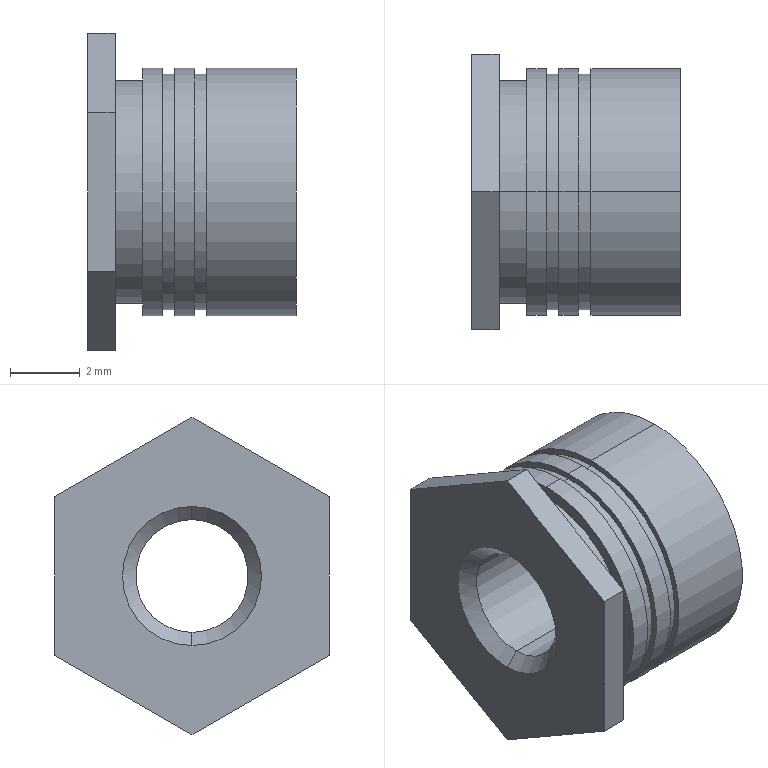Part | NX | features solid 2 | 1 solid | 32 faces | box 6 x 7.9 x 9.122 mm | volume 190.289 mm3 | plane 14 | cylinder 14 | cone 4 | commonest cylinder face diameters 7.12 x6 6.764 x4 3.242 x2 6.408 x2
STEP:
#1=CARTESIAN_POINT('',(-15.92,54.85,-1043.6));
#2=VERTEX_POINT('',#1);
#3=CARTESIAN_POINT('',(-15.92,54.85,-1050.72));
#4=VERTEX_POINT('',#3);
#5=CARTESIAN_POINT('',(-15.92,54.85,-1047.16));
#6=DIRECTION('',(1.,0.,0.));
#7=DIRECTION('',(0.,0.,1.));
#8=AXIS2_PLACEMENT_3D('',#5,#6,#7);
#9=CIRCLE('',#8,3.56);
#10=EDGE_CURVE('',#2,#4,#9,.T.);
#11=ORIENTED_EDGE('',*,*,#10,.F.);
#12=CARTESIAN_POINT('',(-15.92,54.85,-1047.16));
#13=DIRECTION('',(1.,0.,0.));
#14=DIRECTION('',(0.,0.,-1.));
#15=AXIS2_PLACEMENT_3D('',#12,#13,#14);
#16=CIRCLE('',#15,3.56);
#17=EDGE_CURVE('',#4,#2,#16,.T.);
#18=ORIENTED_EDGE('',*,*,#17,.F.);
#19=EDGE_LOOP('',(#11,#18));
#20=FACE_BOUND('',#19,.T.);
#21=CARTESIAN_POINT('',(-15.92,54.85,-1043.956));
#22=VERTEX_POINT('',#21);
#23=CARTESIAN_POINT('',(-15.92,54.85,-1050.364));
#24=VERTEX_POINT('',#23);
#25=CARTESIAN_POINT('',(-15.92,54.85,-1047.16));
#26=DIRECTION('',(-1.,0.,0.));
#27=DIRECTION('',(0.,0.,1.));
#28=AXIS2_PLACEMENT_3D('',#25,#26,#27);
#29=CIRCLE('',#28,3.204);
#30=EDGE_CURVE('',#22,#24,#29,.T.);
#31=ORIENTED_EDGE('',*,*,#30,.F.);
#32=CARTESIAN_POINT('',(-15.92,54.85,-1047.16));
#33=DIRECTION('',(-1.,0.,0.));
#34=DIRECTION('',(0.,0.,-1.));
#35=AXIS2_PLACEMENT_3D('',#32,#33,#34);
#36=CIRCLE('',#35,3.204);
#37=EDGE_CURVE('',#24,#22,#36,.T.);
#38=ORIENTED_EDGE('',*,*,#37,.F.);
#39=EDGE_LOOP('',(#31,#38));
#40=FACE_BOUND('',#39,.T.);
#41=CARTESIAN_POINT('',(-15.92,54.85,-1045.38));
#42=DIRECTION('',(-1.,0.,0.));
#43=DIRECTION('',(0.,1.,0.));
#44=AXIS2_PLACEMENT_3D('',#41,#42,#43);
#45=PLANE('',#44);
#46=ADVANCED_FACE('',(#20,#40),#45,.T.);
#47=CARTESIAN_POINT('',(-15.35,54.85,-1043.6));
#48=VERTEX_POINT('',#47);
#49=CARTESIAN_POINT('',(-15.35,54.85,-1050.72));
#50=VERTEX_POINT('',#49);
#51=CARTESIAN_POINT('',(-15.35,54.85,-1047.16));
#52=DIRECTION('',(-1.,0.,0.));
#53=DIRECTION('',(0.,0.,1.));
#54=AXIS2_PLACEMENT_3D('',#51,#52,#53);
#55=CIRCLE('',#54,3.56);
#56=EDGE_CURVE('',#48,#50,#55,.T.);
#57=ORIENTED_EDGE('',*,*,#56,.T.);
#58=CARTESIAN_POINT('',(-15.92,54.85,-1050.72));
#59=DIRECTION('',(1.,0.,0.));
#60=VECTOR('',#59,1000.);
#61=LINE('',#58,#60);
#62=EDGE_CURVE('',#4,#50,#61,.T.);
#63=ORIENTED_EDGE('',*,*,#62,.F.);
#64=ORIENTED_EDGE('',*,*,#17,.T.);
#65=CARTESIAN_POINT('',(-15.35,54.85,-1043.6));
#66=DIRECTION('',(-1.,0.,0.));
#67=VECTOR('',#66,1000.);
#68=LINE('',#65,#67);
#69=EDGE_CURVE('',#48,#2,#68,.T.);
#70=ORIENTED_EDGE('',*,*,#69,.F.);
#71=EDGE_LOOP('',(#57,#63,#64,#70));
#72=FACE_BOUND('',#71,.T.);
#73=CARTESIAN_POINT('',(-13.71,54.85,-1047.16));
#74=DIRECTION('',(-1.,0.,0.));
#75=DIRECTION('',(0.,0.,-1.));
#76=AXIS2_PLACEMENT_3D('',#73,#74,#75);
#77=CYLINDRICAL_SURFACE('',#76,3.56);
#78=ADVANCED_FACE('',(#72),#77,.T.);
#79=ORIENTED_EDGE('',*,*,#10,.T.);
#80=ORIENTED_EDGE('',*,*,#62,.T.);
#81=CARTESIAN_POINT('',(-15.35,54.85,-1047.16));
#82=DIRECTION('',(-1.,0.,0.));
#83=DIRECTION('',(0.,0.,-1.));
#84=AXIS2_PLACEMENT_3D('',#81,#82,#83);
#85=CIRCLE('',#84,3.56);
#86=EDGE_CURVE('',#50,#48,#85,.T.);
#87=ORIENTED_EDGE('',*,*,#86,.T.);
#88=ORIENTED_EDGE('',*,*,#69,.T.);
#89=EDGE_LOOP('',(#79,#80,#87,#88));
#90=FACE_BOUND('',#89,.T.);
#91=CARTESIAN_POINT('',(-13.71,54.85,-1047.16));
#92=DIRECTION('',(-1.,0.,0.));
#93=DIRECTION('',(0.,0.,-1.));
#94=AXIS2_PLACEMENT_3D('',#91,#92,#93);
#95=CYLINDRICAL_SURFACE('',#94,3.56);
#96=ADVANCED_FACE('',(#90),#95,.T.);
#97=ORIENTED_EDGE('',*,*,#86,.F.);
#98=ORIENTED_EDGE('',*,*,#56,.F.);
#99=EDGE_LOOP('',(#97,#98));
#100=FACE_BOUND('',#99,.T.);
#101=CARTESIAN_POINT('',(-15.35,54.85,-1043.778));
#102=VERTEX_POINT('',#101);
#103=CARTESIAN_POINT('',(-15.35,54.85,-1050.542));
#104=VERTEX_POINT('',#103);
#105=CARTESIAN_POINT('',(-15.35,54.85,-1047.16));
#106=DIRECTION('',(1.,0.,0.));
#107=DIRECTION('',(0.,0.,1.));
#108=AXIS2_PLACEMENT_3D('',#105,#106,#107);
#109=CIRCLE('',#108,3.382);
#110=EDGE_CURVE('',#102,#104,#109,.T.);
#111=ORIENTED_EDGE('',*,*,#110,.F.);
#112=CARTESIAN_POINT('',(-15.35,54.85,-1047.16));
#113=DIRECTION('',(1.,0.,0.));
#114=DIRECTION('',(0.,0.,-1.));
#115=AXIS2_PLACEMENT_3D('',#112,#113,#114);
#116=CIRCLE('',#115,3.382);
#117=EDGE_CURVE('',#104,#102,#116,.T.);
#118=ORIENTED_EDGE('',*,*,#117,.F.);
#119=EDGE_LOOP('',(#111,#118));
#120=FACE_BOUND('',#119,.T.);
#121=CARTESIAN_POINT('',(-15.35,54.85,-1043.689));
#122=DIRECTION('',(-1.,0.,0.));
#123=DIRECTION('',(0.,1.,0.));
#124=AXIS2_PLACEMENT_3D('',#121,#122,#123);
#125=PLANE('',#124);
#126=ADVANCED_FACE('',(#100,#120),#125,.F.);
#127=CARTESIAN_POINT('',(-14.994,54.85,-1043.778));
#128=VERTEX_POINT('',#127);
#129=CARTESIAN_POINT('',(-14.994,54.85,-1050.542));
#130=VERTEX_POINT('',#129);
#131=CARTESIAN_POINT('',(-14.994,54.85,-1047.16));
#132=DIRECTION('',(-1.,0.,0.));
#133=DIRECTION('',(0.,0.,1.));
#134=AXIS2_PLACEMENT_3D('',#131,#132,#133);
#135=CIRCLE('',#134,3.382);
#136=EDGE_CURVE('',#128,#130,#135,.T.);
#137=ORIENTED_EDGE('',*,*,#136,.T.);
#138=CARTESIAN_POINT('',(-14.994,54.85,-1050.542));
#139=DIRECTION('',(-1.,0.,0.));
#140=VECTOR('',#139,1000.);
#141=LINE('',#138,#140);
#142=EDGE_CURVE('',#130,#104,#141,.T.);
#143=ORIENTED_EDGE('',*,*,#142,.T.);
#144=ORIENTED_EDGE('',*,*,#117,.T.);
#145=CARTESIAN_POINT('',(-15.35,54.85,-1043.778));
#146=DIRECTION('',(1.,0.,0.));
#147=VECTOR('',#146,1000.);
#148=LINE('',#145,#147);
#149=EDGE_CURVE('',#102,#128,#148,.T.);
#150=ORIENTED_EDGE('',*,*,#149,.T.);
#151=EDGE_LOOP('',(#137,#143,#144,#150));
#152=FACE_BOUND('',#151,.T.);
#153=CARTESIAN_POINT('',(-15.172,54.85,-1047.16));
#154=DIRECTION('',(-1.,0.,0.));
#155=DIRECTION('',(0.,0.,-1.));
#156=AXIS2_PLACEMENT_3D('',#153,#154,#155);
#157=CYLINDRICAL_SURFACE('',#156,3.382);
#158=ADVANCED_FACE('',(#152),#157,.T.);
#159=ORIENTED_EDGE('',*,*,#110,.T.);
#160=ORIENTED_EDGE('',*,*,#142,.F.);
#161=CARTESIAN_POINT('',(-14.994,54.85,-1047.16));
#162=DIRECTION('',(-1.,0.,0.));
#163=DIRECTION('',(0.,0.,-1.));
#164=AXIS2_PLACEMENT_3D('',#161,#162,#163);
#165=CIRCLE('',#164,3.382);
#166=EDGE_CURVE('',#130,#128,#165,.T.);
#167=ORIENTED_EDGE('',*,*,#166,.T.);
#168=ORIENTED_EDGE('',*,*,#149,.F.);
#169=EDGE_LOOP('',(#159,#160,#167,#168));
#170=FACE_BOUND('',#169,.T.);
#171=CARTESIAN_POINT('',(-15.172,54.85,-1047.16));
#172=DIRECTION('',(-1.,0.,0.));
#173=DIRECTION('',(0.,0.,-1.));
#174=AXIS2_PLACEMENT_3D('',#171,#172,#173);
#175=CYLINDRICAL_SURFACE('',#174,3.382);
#176=ADVANCED_FACE('',(#170),#175,.T.);
#177=CARTESIAN_POINT('',(-14.994,54.85,-1050.72));
#178=VERTEX_POINT('',#177);
#179=CARTESIAN_POINT('',(-14.994,54.85,-1043.6));
#180=VERTEX_POINT('',#179);
#181=CARTESIAN_POINT('',(-14.994,54.85,-1047.16));
#182=DIRECTION('',(1.,0.,0.));
#183=DIRECTION('',(0.,0.,-1.));
#184=AXIS2_PLACEMENT_3D('',#181,#182,#183);
#185=CIRCLE('',#184,3.56);
#186=EDGE_CURVE('',#178,#180,#185,.T.);
#187=ORIENTED_EDGE('',*,*,#186,.F.);
#188=CARTESIAN_POINT('',(-14.994,54.85,-1047.16));
#189=DIRECTION('',(1.,0.,0.));
#190=DIRECTION('',(0.,0.,1.));
#191=AXIS2_PLACEMENT_3D('',#188,#189,#190);
#192=CIRCLE('',#191,3.56);
#193=EDGE_CURVE('',#180,#178,#192,.T.);
#194=ORIENTED_EDGE('',*,*,#193,.F.);
#195=EDGE_LOOP('',(#187,#194));
#196=FACE_BOUND('',#195,.T.);
#197=ORIENTED_EDGE('',*,*,#166,.F.);
#198=ORIENTED_EDGE('',*,*,#136,.F.);
#199=EDGE_LOOP('',(#197,#198));
#200=FACE_BOUND('',#199,.T.);
#201=CARTESIAN_POINT('',(-14.994,54.85,-1043.689));
#202=DIRECTION('',(1.,0.,0.));
#203=DIRECTION('',(0.,1.,0.));
#204=AXIS2_PLACEMENT_3D('',#201,#202,#203);
#205=PLANE('',#204);
#206=ADVANCED_FACE('',(#196,#200),#205,.F.);
#207=ORIENTED_EDGE('',*,*,#193,.T.);
#208=CARTESIAN_POINT('',(-14.425,54.85,-1050.72));
#209=VERTEX_POINT('',#208);
#210=CARTESIAN_POINT('',(-14.994,54.85,-1050.72));
#211=DIRECTION('',(1.,0.,0.));
#212=VECTOR('',#211,1000.);
#213=LINE('',#210,#212);
#214=EDGE_CURVE('',#178,#209,#213,.T.);
#215=ORIENTED_EDGE('',*,*,#214,.T.);
#216=CARTESIAN_POINT('',(-14.425,54.85,-1043.6));
#217=VERTEX_POINT('',#216);
#218=CARTESIAN_POINT('',(-14.425,54.85,-1047.16));
#219=DIRECTION('',(-1.,0.,0.));
#220=DIRECTION('',(0.,0.,-1.));
#221=AXIS2_PLACEMENT_3D('',#218,#219,#220);
#222=CIRCLE('',#221,3.56);
#223=EDGE_CURVE('',#209,#217,#222,.T.);
#224=ORIENTED_EDGE('',*,*,#223,.T.);
#225=CARTESIAN_POINT('',(-14.425,54.85,-1043.6));
#226=DIRECTION('',(-1.,0.,0.));
#227=VECTOR('',#226,1000.);
#228=LINE('',#225,#227);
#229=EDGE_CURVE('',#217,#180,#228,.T.);
#230=ORIENTED_EDGE('',*,*,#229,.T.);
#231=EDGE_LOOP('',(#207,#215,#224,#230));
#232=FACE_BOUND('',#231,.T.);
#233=CARTESIAN_POINT('',(-13.71,54.85,-1047.16));
#234=DIRECTION('',(-1.,0.,0.));
#235=DIRECTION('',(0.,0.,-1.));
#236=AXIS2_PLACEMENT_3D('',#233,#234,#235);
#237=CYLINDRICAL_SURFACE('',#236,3.56);
#238=ADVANCED_FACE('',(#232),#237,.T.);
#239=CARTESIAN_POINT('',(-14.425,54.85,-1047.16));
#240=DIRECTION('',(-1.,0.,0.));
#241=DIRECTION('',(0.,0.,1.));
#242=AXIS2_PLACEMENT_3D('',#239,#240,#241);
#243=CIRCLE('',#242,3.56);
#244=EDGE_CURVE('',#217,#209,#243,.T.);
#245=ORIENTED_EDGE('',*,*,#244,.T.);
#246=ORIENTED_EDGE('',*,*,#214,.F.);
#247=ORIENTED_EDGE('',*,*,#186,.T.);
#248=ORIENTED_EDGE('',*,*,#229,.F.);
#249=EDGE_LOOP('',(#245,#246,#247,#248));
#250=FACE_BOUND('',#249,.T.);
#251=CARTESIAN_POINT('',(-13.71,54.85,-1047.16));
#252=DIRECTION('',(-1.,0.,0.));
#253=DIRECTION('',(0.,0.,-1.));
#254=AXIS2_PLACEMENT_3D('',#251,#252,#253);
#255=CYLINDRICAL_SURFACE('',#254,3.56);
#256=ADVANCED_FACE('',(#250),#255,.T.);
#257=ORIENTED_EDGE('',*,*,#223,.F.);
#258=ORIENTED_EDGE('',*,*,#244,.F.);
#259=EDGE_LOOP('',(#257,#258));
#260=FACE_BOUND('',#259,.T.);
#261=CARTESIAN_POINT('',(-14.425,54.85,-1043.778));
#262=VERTEX_POINT('',#261);
#263=CARTESIAN_POINT('',(-14.425,54.85,-1050.542));
#264=VERTEX_POINT('',#263);
#265=CARTESIAN_POINT('',(-14.425,54.85,-1047.16));
#266=DIRECTION('',(1.,0.,0.));
#267=DIRECTION('',(0.,0.,1.));
#268=AXIS2_PLACEMENT_3D('',#265,#266,#267);
#269=CIRCLE('',#268,3.382);
#270=EDGE_CURVE('',#262,#264,#269,.T.);
#271=ORIENTED_EDGE('',*,*,#270,.F.);
#272=CARTESIAN_POINT('',(-14.425,54.85,-1047.16));
#273=DIRECTION('',(1.,0.,0.));
#274=DIRECTION('',(0.,0.,-1.));
#275=AXIS2_PLACEMENT_3D('',#272,#273,#274);
#276=CIRCLE('',#275,3.382);
#277=EDGE_CURVE('',#264,#262,#276,.T.);
#278=ORIENTED_EDGE('',*,*,#277,.F.);
#279=EDGE_LOOP('',(#271,#278));
#280=FACE_BOUND('',#279,.T.);
#281=CARTESIAN_POINT('',(-14.425,54.85,-1043.689));
#282=DIRECTION('',(-1.,0.,0.));
#283=DIRECTION('',(0.,1.,0.));
#284=AXIS2_PLACEMENT_3D('',#281,#282,#283);
#285=PLANE('',#284);
#286=ADVANCED_FACE('',(#260,#280),#285,.F.);
#287=CARTESIAN_POINT('',(-14.069,54.85,-1043.778));
#288=VERTEX_POINT('',#287);
#289=CARTESIAN_POINT('',(-14.069,54.85,-1050.542));
#290=VERTEX_POINT('',#289);
#291=CARTESIAN_POINT('',(-14.069,54.85,-1047.16));
#292=DIRECTION('',(-1.,0.,0.));
#293=DIRECTION('',(0.,0.,1.));
#294=AXIS2_PLACEMENT_3D('',#291,#292,#293);
#295=CIRCLE('',#294,3.382);
#296=EDGE_CURVE('',#288,#290,#295,.T.);
#297=ORIENTED_EDGE('',*,*,#296,.T.);
#298=CARTESIAN_POINT('',(-14.069,54.85,-1050.542));
#299=DIRECTION('',(-1.,0.,0.));
#300=VECTOR('',#299,1000.);
#301=LINE('',#298,#300);
#302=EDGE_CURVE('',#290,#264,#301,.T.);
#303=ORIENTED_EDGE('',*,*,#302,.T.);
#304=ORIENTED_EDGE('',*,*,#277,.T.);
#305=CARTESIAN_POINT('',(-14.425,54.85,-1043.778));
#306=DIRECTION('',(1.,0.,0.));
#307=VECTOR('',#306,1000.);
#308=LINE('',#305,#307);
#309=EDGE_CURVE('',#262,#288,#308,.T.);
#310=ORIENTED_EDGE('',*,*,#309,.T.);
#311=EDGE_LOOP('',(#297,#303,#304,#310));
#312=FACE_BOUND('',#311,.T.);
#313=CARTESIAN_POINT('',(-14.247,54.85,-1047.16));
#314=DIRECTION('',(-1.,0.,0.));
#315=DIRECTION('',(0.,0.,-1.));
#316=AXIS2_PLACEMENT_3D('',#313,#314,#315);
#317=CYLINDRICAL_SURFACE('',#316,3.382);
#318=ADVANCED_FACE('',(#312),#317,.T.);
#319=ORIENTED_EDGE('',*,*,#270,.T.);
#320=ORIENTED_EDGE('',*,*,#302,.F.);
#321=CARTESIAN_POINT('',(-14.069,54.85,-1047.16));
#322=DIRECTION('',(-1.,0.,0.));
#323=DIRECTION('',(0.,0.,-1.));
#324=AXIS2_PLACEMENT_3D('',#321,#322,#323);
#325=CIRCLE('',#324,3.382);
#326=EDGE_CURVE('',#290,#288,#325,.T.);
#327=ORIENTED_EDGE('',*,*,#326,.T.);
#328=ORIENTED_EDGE('',*,*,#309,.F.);
#329=EDGE_LOOP('',(#319,#320,#327,#328));
#330=FACE_BOUND('',#329,.T.);
#331=CARTESIAN_POINT('',(-14.247,54.85,-1047.16));
#332=DIRECTION('',(-1.,0.,0.));
#333=DIRECTION('',(0.,0.,-1.));
#334=AXIS2_PLACEMENT_3D('',#331,#332,#333);
#335=CYLINDRICAL_SURFACE('',#334,3.382);
#336=ADVANCED_FACE('',(#330),#335,.T.);
#337=CARTESIAN_POINT('',(-14.069,54.85,-1050.72));
#338=VERTEX_POINT('',#337);
#339=CARTESIAN_POINT('',(-14.069,54.85,-1043.6));
#340=VERTEX_POINT('',#339);
#341=CARTESIAN_POINT('',(-14.069,54.85,-1047.16));
#342=DIRECTION('',(1.,0.,0.));
#343=DIRECTION('',(0.,0.,-1.));
#344=AXIS2_PLACEMENT_3D('',#341,#342,#343);
#345=CIRCLE('',#344,3.56);
#346=EDGE_CURVE('',#338,#340,#345,.T.);
#347=ORIENTED_EDGE('',*,*,#346,.F.);
#348=CARTESIAN_POINT('',(-14.069,54.85,-1047.16));
#349=DIRECTION('',(1.,0.,0.));
#350=DIRECTION('',(0.,0.,1.));
#351=AXIS2_PLACEMENT_3D('',#348,#349,#350);
#352=CIRCLE('',#351,3.56);
#353=EDGE_CURVE('',#340,#338,#352,.T.);
#354=ORIENTED_EDGE('',*,*,#353,.F.);
#355=EDGE_LOOP('',(#347,#354));
#356=FACE_BOUND('',#355,.T.);
#357=ORIENTED_EDGE('',*,*,#326,.F.);
#358=ORIENTED_EDGE('',*,*,#296,.F.);
#359=EDGE_LOOP('',(#357,#358));
#360=FACE_BOUND('',#359,.T.);
#361=CARTESIAN_POINT('',(-14.069,54.85,-1043.689));
#362=DIRECTION('',(1.,0.,0.));
#363=DIRECTION('',(0.,1.,0.));
#364=AXIS2_PLACEMENT_3D('',#361,#362,#363);
#365=PLANE('',#364);
#366=ADVANCED_FACE('',(#356,#360),#365,.F.);
#367=ORIENTED_EDGE('',*,*,#353,.T.);
#368=CARTESIAN_POINT('',(-11.5,54.85,-1050.72));
#369=VERTEX_POINT('',#368);
#370=CARTESIAN_POINT('',(-14.069,54.85,-1050.72));
#371=DIRECTION('',(1.,0.,0.));
#372=VECTOR('',#371,1000.);
#373=LINE('',#370,#372);
#374=EDGE_CURVE('',#338,#369,#373,.T.);
#375=ORIENTED_EDGE('',*,*,#374,.T.);
#376=CARTESIAN_POINT('',(-11.5,54.85,-1043.6));
#377=VERTEX_POINT('',#376);
#378=CARTESIAN_POINT('',(-11.5,54.85,-1047.16));
#379=DIRECTION('',(-1.,0.,0.));
#380=DIRECTION('',(0.,0.,-1.));
#381=AXIS2_PLACEMENT_3D('',#378,#379,#380);
#382=CIRCLE('',#381,3.56);
#383=EDGE_CURVE('',#369,#377,#382,.T.);
#384=ORIENTED_EDGE('',*,*,#383,.T.);
#385=CARTESIAN_POINT('',(-11.5,54.85,-1043.6));
#386=DIRECTION('',(-1.,0.,0.));
#387=VECTOR('',#386,1000.);
#388=LINE('',#385,#387);
#389=EDGE_CURVE('',#377,#340,#388,.T.);
#390=ORIENTED_EDGE('',*,*,#389,.T.);
#391=EDGE_LOOP('',(#367,#375,#384,#390));
#392=FACE_BOUND('',#391,.T.);
#393=CARTESIAN_POINT('',(-13.71,54.85,-1047.16));
#394=DIRECTION('',(-1.,0.,0.));
#395=DIRECTION('',(0.,0.,-1.));
#396=AXIS2_PLACEMENT_3D('',#393,#394,#395);
#397=CYLINDRICAL_SURFACE('',#396,3.56);
#398=ADVANCED_FACE('',(#392),#397,.T.);
#399=CARTESIAN_POINT('',(-11.5,54.85,-1047.16));
#400=DIRECTION('',(-1.,0.,0.));
#401=DIRECTION('',(0.,0.,1.));
#402=AXIS2_PLACEMENT_3D('',#399,#400,#401);
#403=CIRCLE('',#402,3.56);
#404=EDGE_CURVE('',#377,#369,#403,.T.);
#405=ORIENTED_EDGE('',*,*,#404,.T.);
#406=ORIENTED_EDGE('',*,*,#374,.F.);
#407=ORIENTED_EDGE('',*,*,#346,.T.);
#408=ORIENTED_EDGE('',*,*,#389,.F.);
#409=EDGE_LOOP('',(#405,#406,#407,#408));
#410=FACE_BOUND('',#409,.T.);
#411=CARTESIAN_POINT('',(-13.71,54.85,-1047.16));
#412=DIRECTION('',(-1.,0.,0.));
#413=DIRECTION('',(0.,0.,-1.));
#414=AXIS2_PLACEMENT_3D('',#411,#412,#413);
#415=CYLINDRICAL_SURFACE('',#414,3.56);
#416=ADVANCED_FACE('',(#410),#415,.T.);
#417=ORIENTED_EDGE('',*,*,#383,.F.);
#418=ORIENTED_EDGE('',*,*,#404,.F.);
#419=EDGE_LOOP('',(#417,#418));
#420=FACE_BOUND('',#419,.T.);
#421=CARTESIAN_POINT('',(-11.5,54.85,-1045.16));
#422=VERTEX_POINT('',#421);
#423=CARTESIAN_POINT('',(-11.5,54.85,-1049.16));
#424=VERTEX_POINT('',#423);
#425=CARTESIAN_POINT('',(-11.5,54.85,-1047.16));
#426=DIRECTION('',(1.,0.,0.));
#427=DIRECTION('',(0.,0.,1.));
#428=AXIS2_PLACEMENT_3D('',#425,#426,#427);
#429=CIRCLE('',#428,2.);
#430=EDGE_CURVE('',#422,#424,#429,.T.);
#431=ORIENTED_EDGE('',*,*,#430,.F.);
#432=CARTESIAN_POINT('',(-11.5,54.85,-1047.16));
#433=DIRECTION('',(1.,0.,0.));
#434=DIRECTION('',(0.,0.,-1.));
#435=AXIS2_PLACEMENT_3D('',#432,#433,#434);
#436=CIRCLE('',#435,2.);
#437=EDGE_CURVE('',#424,#422,#436,.T.);
#438=ORIENTED_EDGE('',*,*,#437,.F.);
#439=EDGE_LOOP('',(#431,#438));
#440=FACE_BOUND('',#439,.T.);
#441=CARTESIAN_POINT('',(-11.5,54.85,-1045.38));
#442=DIRECTION('',(1.,0.,0.));
#443=DIRECTION('',(0.,1.,0.));
#444=AXIS2_PLACEMENT_3D('',#441,#442,#443);
#445=PLANE('',#444);
#446=ADVANCED_FACE('',(#420,#440),#445,.T.);
#447=ORIENTED_EDGE('',*,*,#437,.T.);
#448=CARTESIAN_POINT('',(-11.879,54.85,-1045.539));
#449=VERTEX_POINT('',#448);
#450=CARTESIAN_POINT('',(-11.879,54.85,-1045.539));
#451=DIRECTION('',(0.7071,0.,0.7071));
#452=VECTOR('',#451,1000.);
#453=LINE('',#450,#452);
#454=EDGE_CURVE('',#449,#422,#453,.T.);
#455=ORIENTED_EDGE('',*,*,#454,.F.);
#456=CARTESIAN_POINT('',(-11.879,54.85,-1048.781));
#457=VERTEX_POINT('',#456);
#458=CARTESIAN_POINT('',(-11.879,54.85,-1047.16));
#459=DIRECTION('',(1.,0.,0.));
#460=DIRECTION('',(0.,0.,-1.));
#461=AXIS2_PLACEMENT_3D('',#458,#459,#460);
#462=CIRCLE('',#461,1.621);
#463=EDGE_CURVE('',#457,#449,#462,.T.);
#464=ORIENTED_EDGE('',*,*,#463,.F.);
#465=CARTESIAN_POINT('',(-11.5,54.85,-1049.16));
#466=DIRECTION('',(-0.7071,0.,0.7071));
#467=VECTOR('',#466,1000.);
#468=LINE('',#465,#467);
#469=EDGE_CURVE('',#424,#457,#468,.T.);
#470=ORIENTED_EDGE('',*,*,#469,.F.);
#471=EDGE_LOOP('',(#447,#455,#464,#470));
#472=FACE_BOUND('',#471,.T.);
#473=CARTESIAN_POINT('',(-11.69,54.85,-1047.16));
#474=DIRECTION('',(1.,0.,0.));
#475=DIRECTION('',(0.,0.,1.));
#476=AXIS2_PLACEMENT_3D('',#473,#474,#475);
#477=CONICAL_SURFACE('',#476,1.81,0.7854);
#478=ADVANCED_FACE('',(#472),#477,.F.);
#479=CARTESIAN_POINT('',(-11.879,54.85,-1047.16));
#480=DIRECTION('',(1.,0.,0.));
#481=DIRECTION('',(0.,0.,1.));
#482=AXIS2_PLACEMENT_3D('',#479,#480,#481);
#483=CIRCLE('',#482,1.621);
#484=EDGE_CURVE('',#449,#457,#483,.T.);
#485=ORIENTED_EDGE('',*,*,#484,.F.);
#486=ORIENTED_EDGE('',*,*,#454,.T.);
#487=ORIENTED_EDGE('',*,*,#430,.T.);
#488=ORIENTED_EDGE('',*,*,#469,.T.);
#489=EDGE_LOOP('',(#485,#486,#487,#488));
#490=FACE_BOUND('',#489,.T.);
#491=CARTESIAN_POINT('',(-11.69,54.85,-1047.16));
#492=DIRECTION('',(1.,0.,0.));
#493=DIRECTION('',(0.,0.,1.));
#494=AXIS2_PLACEMENT_3D('',#491,#492,#493);
#495=CONICAL_SURFACE('',#494,1.81,0.7854);
#496=ADVANCED_FACE('',(#490),#495,.F.);
#497=CARTESIAN_POINT('',(-17.121,54.85,-1048.781));
#498=VERTEX_POINT('',#497);
#499=CARTESIAN_POINT('',(-17.121,54.85,-1045.539));
#500=VERTEX_POINT('',#499);
#501=CARTESIAN_POINT('',(-17.121,54.85,-1047.16));
#502=DIRECTION('',(-1.,0.,0.));
#503=DIRECTION('',(0.,0.,-1.));
#504=AXIS2_PLACEMENT_3D('',#501,#502,#503);
#505=CIRCLE('',#504,1.621);
#506=EDGE_CURVE('',#498,#500,#505,.T.);
#507=ORIENTED_EDGE('',*,*,#506,.T.);
#508=CARTESIAN_POINT('',(-17.121,54.85,-1045.539));
#509=DIRECTION('',(1.,0.,0.));
#510=VECTOR('',#509,1000.);
#511=LINE('',#508,#510);
#512=EDGE_CURVE('',#500,#449,#511,.T.);
#513=ORIENTED_EDGE('',*,*,#512,.T.);
#514=ORIENTED_EDGE('',*,*,#484,.T.);
#515=CARTESIAN_POINT('',(-11.879,54.85,-1048.781));
#516=DIRECTION('',(-1.,0.,0.));
#517=VECTOR('',#516,1000.);
#518=LINE('',#515,#517);
#519=EDGE_CURVE('',#457,#498,#518,.T.);
#520=ORIENTED_EDGE('',*,*,#519,.T.);
#521=EDGE_LOOP('',(#507,#513,#514,#520));
#522=FACE_BOUND('',#521,.T.);
#523=CARTESIAN_POINT('',(-14.5,54.85,-1047.16));
#524=DIRECTION('',(-1.,0.,0.));
#525=DIRECTION('',(0.,0.,1.));
#526=AXIS2_PLACEMENT_3D('',#523,#524,#525);
#527=CYLINDRICAL_SURFACE('',#526,1.621);
#528=ADVANCED_FACE('',(#522),#527,.F.);
#529=ORIENTED_EDGE('',*,*,#463,.T.);
#530=ORIENTED_EDGE('',*,*,#512,.F.);
#531=CARTESIAN_POINT('',(-17.121,54.85,-1047.16));
#532=DIRECTION('',(-1.,0.,0.));
#533=DIRECTION('',(0.,0.,1.));
#534=AXIS2_PLACEMENT_3D('',#531,#532,#533);
#535=CIRCLE('',#534,1.621);
#536=EDGE_CURVE('',#500,#498,#535,.T.);
#537=ORIENTED_EDGE('',*,*,#536,.T.);
#538=ORIENTED_EDGE('',*,*,#519,.F.);
#539=EDGE_LOOP('',(#529,#530,#537,#538));
#540=FACE_BOUND('',#539,.T.);
#541=CARTESIAN_POINT('',(-14.5,54.85,-1047.16));
#542=DIRECTION('',(-1.,0.,0.));
#543=DIRECTION('',(0.,0.,1.));
#544=AXIS2_PLACEMENT_3D('',#541,#542,#543);
#545=CYLINDRICAL_SURFACE('',#544,1.621);
#546=ADVANCED_FACE('',(#540),#545,.F.);
#547=ORIENTED_EDGE('',*,*,#536,.F.);
#548=CARTESIAN_POINT('',(-17.5,54.85,-1045.16));
#549=VERTEX_POINT('',#548);
#550=CARTESIAN_POINT('',(-17.5,54.85,-1045.16));
#551=DIRECTION('',(0.7071,0.,-0.7071));
#552=VECTOR('',#551,1000.);
#553=LINE('',#550,#552);
#554=EDGE_CURVE('',#549,#500,#553,.T.);
#555=ORIENTED_EDGE('',*,*,#554,.F.);
#556=CARTESIAN_POINT('',(-17.5,54.85,-1049.16));
#557=VERTEX_POINT('',#556);
#558=CARTESIAN_POINT('',(-17.5,54.85,-1047.16));
#559=DIRECTION('',(-1.,0.,0.));
#560=DIRECTION('',(0.,0.,1.));
#561=AXIS2_PLACEMENT_3D('',#558,#559,#560);
#562=CIRCLE('',#561,2.);
#563=EDGE_CURVE('',#549,#557,#562,.T.);
#564=ORIENTED_EDGE('',*,*,#563,.T.);
#565=CARTESIAN_POINT('',(-17.121,54.85,-1048.781));
#566=DIRECTION('',(-0.7071,0.,-0.7071));
#567=VECTOR('',#566,1000.);
#568=LINE('',#565,#567);
#569=EDGE_CURVE('',#498,#557,#568,.T.);
#570=ORIENTED_EDGE('',*,*,#569,.F.);
#571=EDGE_LOOP('',(#547,#555,#564,#570));
#572=FACE_BOUND('',#571,.T.);
#573=CARTESIAN_POINT('',(-17.311,54.85,-1047.16));
#574=DIRECTION('',(-1.,0.,0.));
#575=DIRECTION('',(0.,0.,1.));
#576=AXIS2_PLACEMENT_3D('',#573,#574,#575);
#577=CONICAL_SURFACE('',#576,1.81,0.7854);
#578=ADVANCED_FACE('',(#572),#577,.F.);
#579=CARTESIAN_POINT('',(-17.5,54.85,-1047.16));
#580=DIRECTION('',(-1.,0.,0.));
#581=DIRECTION('',(0.,0.,-1.));
#582=AXIS2_PLACEMENT_3D('',#579,#580,#581);
#583=CIRCLE('',#582,2.);
#584=EDGE_CURVE('',#557,#549,#583,.T.);
#585=ORIENTED_EDGE('',*,*,#584,.T.);
#586=ORIENTED_EDGE('',*,*,#554,.T.);
#587=ORIENTED_EDGE('',*,*,#506,.F.);
#588=ORIENTED_EDGE('',*,*,#569,.T.);
#589=EDGE_LOOP('',(#585,#586,#587,#588));
#590=FACE_BOUND('',#589,.T.);
#591=CARTESIAN_POINT('',(-17.311,54.85,-1047.16));
#592=DIRECTION('',(-1.,0.,0.));
#593=DIRECTION('',(0.,0.,1.));
#594=AXIS2_PLACEMENT_3D('',#591,#592,#593);
#595=CONICAL_SURFACE('',#594,1.81,0.7854);
#596=ADVANCED_FACE('',(#590),#595,.F.);
#597=CARTESIAN_POINT('',(-17.5,54.85,-1042.599));
#598=VERTEX_POINT('',#597);
#599=CARTESIAN_POINT('',(-17.5,50.9,-1044.879));
#600=VERTEX_POINT('',#599);
#601=CARTESIAN_POINT('',(-17.5,54.85,-1042.599));
#602=DIRECTION('',(0.,-0.866,-0.5));
#603=VECTOR('',#602,1000.);
#604=LINE('',#601,#603);
#605=EDGE_CURVE('',#598,#600,#604,.T.);
#606=ORIENTED_EDGE('',*,*,#605,.F.);
#607=CARTESIAN_POINT('',(-17.5,58.8,-1044.879));
#608=VERTEX_POINT('',#607);
#609=CARTESIAN_POINT('',(-17.5,58.8,-1044.879));
#610=DIRECTION('',(0.,-0.866,0.5));
#611=VECTOR('',#610,1000.);
#612=LINE('',#609,#611);
#613=EDGE_CURVE('',#608,#598,#612,.T.);
#614=ORIENTED_EDGE('',*,*,#613,.F.);
#615=CARTESIAN_POINT('',(-17.5,58.8,-1049.441));
#616=VERTEX_POINT('',#615);
#617=CARTESIAN_POINT('',(-17.5,58.8,-1049.441));
#618=DIRECTION('',(0.,0.,1.));
#619=VECTOR('',#618,1000.);
#620=LINE('',#617,#619);
#621=EDGE_CURVE('',#616,#608,#620,.T.);
#622=ORIENTED_EDGE('',*,*,#621,.F.);
#623=CARTESIAN_POINT('',(-17.5,54.85,-1051.721));
#624=VERTEX_POINT('',#623);
#625=CARTESIAN_POINT('',(-17.5,54.85,-1051.721));
#626=DIRECTION('',(0.,0.866,0.5));
#627=VECTOR('',#626,1000.);
#628=LINE('',#625,#627);
#629=EDGE_CURVE('',#624,#616,#628,.T.);
#630=ORIENTED_EDGE('',*,*,#629,.F.);
#631=CARTESIAN_POINT('',(-17.5,50.9,-1049.441));
#632=VERTEX_POINT('',#631);
#633=CARTESIAN_POINT('',(-17.5,50.9,-1049.441));
#634=DIRECTION('',(0.,0.866,-0.5));
#635=VECTOR('',#634,1000.);
#636=LINE('',#633,#635);
#637=EDGE_CURVE('',#632,#624,#636,.T.);
#638=ORIENTED_EDGE('',*,*,#637,.F.);
#639=CARTESIAN_POINT('',(-17.5,50.9,-1044.879));
#640=DIRECTION('',(0.,0.,-1.));
#641=VECTOR('',#640,1000.);
#642=LINE('',#639,#641);
#643=EDGE_CURVE('',#600,#632,#642,.T.);
#644=ORIENTED_EDGE('',*,*,#643,.F.);
#645=EDGE_LOOP('',(#606,#614,#622,#630,#638,#644));
#646=FACE_BOUND('',#645,.T.);
#647=ORIENTED_EDGE('',*,*,#563,.F.);
#648=ORIENTED_EDGE('',*,*,#584,.F.);
#649=EDGE_LOOP('',(#647,#648));
#650=FACE_BOUND('',#649,.T.);
#651=CARTESIAN_POINT('',(-17.5,54.85,-1047.16));
#652=DIRECTION('',(-1.,0.,0.));
#653=DIRECTION('',(0.,1.,0.));
#654=AXIS2_PLACEMENT_3D('',#651,#652,#653);
#655=PLANE('',#654);
#656=ADVANCED_FACE('',(#646,#650),#655,.T.);
#657=CARTESIAN_POINT('',(-16.71,50.9,-1049.441));
#658=VERTEX_POINT('',#657);
#659=CARTESIAN_POINT('',(-16.71,50.9,-1049.441));
#660=DIRECTION('',(-1.,0.,0.));
#661=VECTOR('',#660,1000.);
#662=LINE('',#659,#661);
#663=EDGE_CURVE('',#658,#632,#662,.T.);
#664=ORIENTED_EDGE('',*,*,#663,.F.);
#665=CARTESIAN_POINT('',(-16.71,50.9,-1044.879));
#666=VERTEX_POINT('',#665);
#667=CARTESIAN_POINT('',(-16.71,50.9,-1049.441));
#668=DIRECTION('',(0.,0.,1.));
#669=VECTOR('',#668,1000.);
#670=LINE('',#667,#669);
#671=EDGE_CURVE('',#658,#666,#670,.T.);
#672=ORIENTED_EDGE('',*,*,#671,.T.);
#673=CARTESIAN_POINT('',(-16.71,50.9,-1044.879));
#674=DIRECTION('',(-1.,0.,0.));
#675=VECTOR('',#674,1000.);
#676=LINE('',#673,#675);
#677=EDGE_CURVE('',#666,#600,#676,.T.);
#678=ORIENTED_EDGE('',*,*,#677,.T.);
#679=ORIENTED_EDGE('',*,*,#643,.T.);
#680=EDGE_LOOP('',(#664,#672,#678,#679));
#681=FACE_BOUND('',#680,.T.);
#682=CARTESIAN_POINT('',(-16.71,50.9,-1044.879));
#683=DIRECTION('',(0.,-1.,0.));
#684=DIRECTION('',(1.,0.,0.));
#685=AXIS2_PLACEMENT_3D('',#682,#683,#684);
#686=PLANE('',#685);
#687=ADVANCED_FACE('',(#681),#686,.T.);
#688=ORIENTED_EDGE('',*,*,#677,.F.);
#689=CARTESIAN_POINT('',(-16.71,54.85,-1042.599));
#690=VERTEX_POINT('',#689);
#691=CARTESIAN_POINT('',(-16.71,50.9,-1044.879));
#692=DIRECTION('',(0.,0.866,0.5));
#693=VECTOR('',#692,1000.);
#694=LINE('',#691,#693);
#695=EDGE_CURVE('',#666,#690,#694,.T.);
#696=ORIENTED_EDGE('',*,*,#695,.T.);
#697=CARTESIAN_POINT('',(-16.71,54.85,-1042.599));
#698=DIRECTION('',(-1.,0.,0.));
#699=VECTOR('',#698,1000.);
#700=LINE('',#697,#699);
#701=EDGE_CURVE('',#690,#598,#700,.T.);
#702=ORIENTED_EDGE('',*,*,#701,.T.);
#703=ORIENTED_EDGE('',*,*,#605,.T.);
#704=EDGE_LOOP('',(#688,#696,#702,#703));
#705=FACE_BOUND('',#704,.T.);
#706=CARTESIAN_POINT('',(-16.71,54.85,-1042.599));
#707=DIRECTION('',(0.,-0.5,0.866));
#708=DIRECTION('',(1.,0.,0.));
#709=AXIS2_PLACEMENT_3D('',#706,#707,#708);
#710=PLANE('',#709);
#711=ADVANCED_FACE('',(#705),#710,.T.);
#712=ORIENTED_EDGE('',*,*,#701,.F.);
#713=CARTESIAN_POINT('',(-16.71,58.8,-1044.879));
#714=VERTEX_POINT('',#713);
#715=CARTESIAN_POINT('',(-16.71,54.85,-1042.599));
#716=DIRECTION('',(0.,0.866,-0.5));
#717=VECTOR('',#716,1000.);
#718=LINE('',#715,#717);
#719=EDGE_CURVE('',#690,#714,#718,.T.);
#720=ORIENTED_EDGE('',*,*,#719,.T.);
#721=CARTESIAN_POINT('',(-16.71,58.8,-1044.879));
#722=DIRECTION('',(-1.,0.,0.));
#723=VECTOR('',#722,1000.);
#724=LINE('',#721,#723);
#725=EDGE_CURVE('',#714,#608,#724,.T.);
#726=ORIENTED_EDGE('',*,*,#725,.T.);
#727=ORIENTED_EDGE('',*,*,#613,.T.);
#728=EDGE_LOOP('',(#712,#720,#726,#727));
#729=FACE_BOUND('',#728,.T.);
#730=CARTESIAN_POINT('',(-16.71,58.8,-1044.879));
#731=DIRECTION('',(0.,0.5,0.866));
#732=DIRECTION('',(1.,0.,0.));
#733=AXIS2_PLACEMENT_3D('',#730,#731,#732);
#734=PLANE('',#733);
#735=ADVANCED_FACE('',(#729),#734,.T.);
#736=ORIENTED_EDGE('',*,*,#725,.F.);
#737=CARTESIAN_POINT('',(-16.71,58.8,-1049.441));
#738=VERTEX_POINT('',#737);
#739=CARTESIAN_POINT('',(-16.71,58.8,-1044.879));
#740=DIRECTION('',(0.,0.,-1.));
#741=VECTOR('',#740,1000.);
#742=LINE('',#739,#741);
#743=EDGE_CURVE('',#714,#738,#742,.T.);
#744=ORIENTED_EDGE('',*,*,#743,.T.);
#745=CARTESIAN_POINT('',(-16.71,58.8,-1049.441));
#746=DIRECTION('',(-1.,0.,0.));
#747=VECTOR('',#746,1000.);
#748=LINE('',#745,#747);
#749=EDGE_CURVE('',#738,#616,#748,.T.);
#750=ORIENTED_EDGE('',*,*,#749,.T.);
#751=ORIENTED_EDGE('',*,*,#621,.T.);
#752=EDGE_LOOP('',(#736,#744,#750,#751));
#753=FACE_BOUND('',#752,.T.);
#754=CARTESIAN_POINT('',(-16.71,58.8,-1049.441));
#755=DIRECTION('',(0.,1.,0.));
#756=DIRECTION('',(1.,0.,0.));
#757=AXIS2_PLACEMENT_3D('',#754,#755,#756);
#758=PLANE('',#757);
#759=ADVANCED_FACE('',(#753),#758,.T.);
#760=ORIENTED_EDGE('',*,*,#749,.F.);
#761=CARTESIAN_POINT('',(-16.71,54.85,-1051.721));
#762=VERTEX_POINT('',#761);
#763=CARTESIAN_POINT('',(-16.71,58.8,-1049.441));
#764=DIRECTION('',(0.,-0.866,-0.5));
#765=VECTOR('',#764,1000.);
#766=LINE('',#763,#765);
#767=EDGE_CURVE('',#738,#762,#766,.T.);
#768=ORIENTED_EDGE('',*,*,#767,.T.);
#769=CARTESIAN_POINT('',(-16.71,54.85,-1051.721));
#770=DIRECTION('',(-1.,0.,0.));
#771=VECTOR('',#770,1000.);
#772=LINE('',#769,#771);
#773=EDGE_CURVE('',#762,#624,#772,.T.);
#774=ORIENTED_EDGE('',*,*,#773,.T.);
#775=ORIENTED_EDGE('',*,*,#629,.T.);
#776=EDGE_LOOP('',(#760,#768,#774,#775));
#777=FACE_BOUND('',#776,.T.);
#778=CARTESIAN_POINT('',(-16.71,54.85,-1051.721));
#779=DIRECTION('',(0.,0.5,-0.866));
#780=DIRECTION('',(1.,0.,0.));
#781=AXIS2_PLACEMENT_3D('',#778,#779,#780);
#782=PLANE('',#781);
#783=ADVANCED_FACE('',(#777),#782,.T.);
#784=ORIENTED_EDGE('',*,*,#773,.F.);
#785=CARTESIAN_POINT('',(-16.71,54.85,-1051.721));
#786=DIRECTION('',(0.,-0.866,0.5));
#787=VECTOR('',#786,1000.);
#788=LINE('',#785,#787);
#789=EDGE_CURVE('',#762,#658,#788,.T.);
#790=ORIENTED_EDGE('',*,*,#789,.T.);
#791=ORIENTED_EDGE('',*,*,#663,.T.);
#792=ORIENTED_EDGE('',*,*,#637,.T.);
#793=EDGE_LOOP('',(#784,#790,#791,#792));
#794=FACE_BOUND('',#793,.T.);
#795=CARTESIAN_POINT('',(-16.71,50.9,-1049.441));
#796=DIRECTION('',(0.,-0.5,-0.866));
#797=DIRECTION('',(1.,0.,0.));
#798=AXIS2_PLACEMENT_3D('',#795,#796,#797);
#799=PLANE('',#798);
#800=ADVANCED_FACE('',(#794),#799,.T.);
#801=ORIENTED_EDGE('',*,*,#671,.F.);
#802=ORIENTED_EDGE('',*,*,#789,.F.);
#803=ORIENTED_EDGE('',*,*,#767,.F.);
#804=ORIENTED_EDGE('',*,*,#743,.F.);
#805=ORIENTED_EDGE('',*,*,#719,.F.);
#806=ORIENTED_EDGE('',*,*,#695,.F.);
#807=EDGE_LOOP('',(#801,#802,#803,#804,#805,#806));
#808=FACE_BOUND('',#807,.T.);
#809=CARTESIAN_POINT('',(-16.71,54.85,-1043.956));
#810=VERTEX_POINT('',#809);
#811=CARTESIAN_POINT('',(-16.71,54.85,-1050.364));
#812=VERTEX_POINT('',#811);
#813=CARTESIAN_POINT('',(-16.71,54.85,-1047.16));
#814=DIRECTION('',(1.,0.,0.));
#815=DIRECTION('',(0.,0.,1.));
#816=AXIS2_PLACEMENT_3D('',#813,#814,#815);
#817=CIRCLE('',#816,3.204);
#818=EDGE_CURVE('',#810,#812,#817,.T.);
#819=ORIENTED_EDGE('',*,*,#818,.F.);
#820=CARTESIAN_POINT('',(-16.71,54.85,-1047.16));
#821=DIRECTION('',(1.,0.,0.));
#822=DIRECTION('',(0.,0.,-1.));
#823=AXIS2_PLACEMENT_3D('',#820,#821,#822);
#824=CIRCLE('',#823,3.204);
#825=EDGE_CURVE('',#812,#810,#824,.T.);
#826=ORIENTED_EDGE('',*,*,#825,.F.);
#827=EDGE_LOOP('',(#819,#826));
#828=FACE_BOUND('',#827,.T.);
#829=CARTESIAN_POINT('',(-16.71,54.85,-1047.16));
#830=DIRECTION('',(-1.,0.,0.));
#831=DIRECTION('',(0.,1.,0.));
#832=AXIS2_PLACEMENT_3D('',#829,#830,#831);
#833=PLANE('',#832);
#834=ADVANCED_FACE('',(#808,#828),#833,.F.);
#835=ORIENTED_EDGE('',*,*,#30,.T.);
#836=CARTESIAN_POINT('',(-16.71,54.85,-1050.364));
#837=DIRECTION('',(1.,0.,0.));
#838=VECTOR('',#837,1000.);
#839=LINE('',#836,#838);
#840=EDGE_CURVE('',#812,#24,#839,.T.);
#841=ORIENTED_EDGE('',*,*,#840,.F.);
#842=ORIENTED_EDGE('',*,*,#825,.T.);
#843=CARTESIAN_POINT('',(-15.92,54.85,-1043.956));
#844=DIRECTION('',(-1.,0.,0.));
#845=VECTOR('',#844,1000.);
#846=LINE('',#843,#845);
#847=EDGE_CURVE('',#22,#810,#846,.T.);
#848=ORIENTED_EDGE('',*,*,#847,.F.);
#849=EDGE_LOOP('',(#835,#841,#842,#848));
#850=FACE_BOUND('',#849,.T.);
#851=CARTESIAN_POINT('',(-16.315,54.85,-1047.16));
#852=DIRECTION('',(-1.,0.,0.));
#853=DIRECTION('',(0.,0.,-1.));
#854=AXIS2_PLACEMENT_3D('',#851,#852,#853);
#855=CYLINDRICAL_SURFACE('',#854,3.204);
#856=ADVANCED_FACE('',(#850),#855,.T.);
#857=ORIENTED_EDGE('',*,*,#818,.T.);
#858=ORIENTED_EDGE('',*,*,#840,.T.);
#859=ORIENTED_EDGE('',*,*,#37,.T.);
#860=ORIENTED_EDGE('',*,*,#847,.T.);
#861=EDGE_LOOP('',(#857,#858,#859,#860));
#862=FACE_BOUND('',#861,.T.);
#863=CARTESIAN_POINT('',(-16.315,54.85,-1047.16));
#864=DIRECTION('',(-1.,0.,0.));
#865=DIRECTION('',(0.,0.,-1.));
#866=AXIS2_PLACEMENT_3D('',#863,#864,#865);
#867=CYLINDRICAL_SURFACE('',#866,3.204);
#868=ADVANCED_FACE('',(#862),#867,.T.);
#869=CLOSED_SHELL('',(#46,#78,#96,#126,#158,#176,#206,#238,#256,#286,#318,#336,#366,#398,#416,#446,#478,#496,#528,#546,#578,#596,#656,#687,#711,#735,#759,#783,#800,#834,#856,#868));
#870=MANIFOLD_SOLID_BREP('',#869);
#871=(LENGTH_UNIT()NAMED_UNIT(*)SI_UNIT(.MILLI.,.METRE.));
#872=UNCERTAINTY_MEASURE_WITH_UNIT(LENGTH_MEASURE(0.00001),#871,'','');
#873=(NAMED_UNIT(*)PLANE_ANGLE_UNIT()SI_UNIT($,.RADIAN.));
#874=(NAMED_UNIT(*)SI_UNIT($,.STERADIAN.)SOLID_ANGLE_UNIT());
#875=(GEOMETRIC_REPRESENTATION_CONTEXT(3)GLOBAL_UNCERTAINTY_ASSIGNED_CONTEXT((#872))GLOBAL_UNIT_ASSIGNED_CONTEXT((#871,#873,#874))REPRESENTATION_CONTEXT('',''));
#876=ADVANCED_BREP_SHAPE_REPRESENTATION('',(#870),#875);